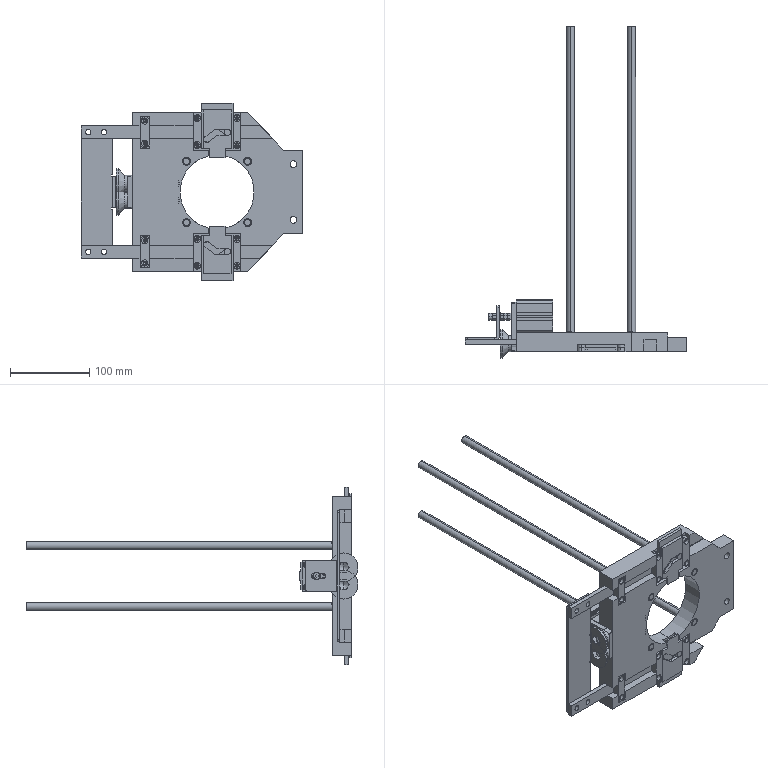Part | SolidWorks | 32 solids | 1039 faces | box 279.24 x 418.025 x 223.859 mm | volume 966328 mm3 | cylinder 501 | plane 388 | cone 124 | spline 26 | commonest cylinder face diameters 10 x172 5 x70 8 x44 3.3 x24 4.5 x24 8.5 x22